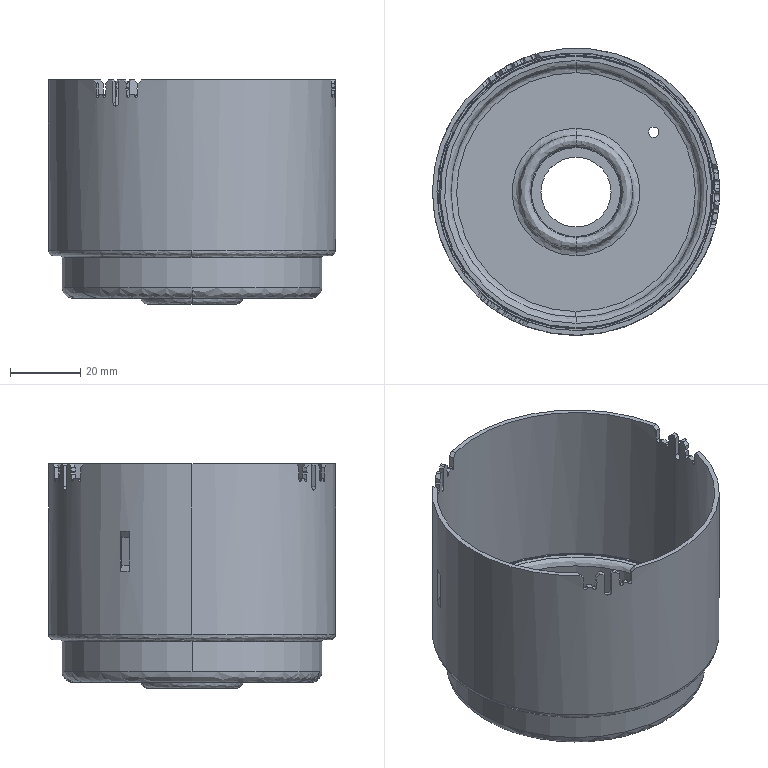Part | STEP file | TQ-DD-1105-THA140062100B_Housing1010_デフォルト | 1 solid | 157 faces | box 82 x 82 x 64.1 mm | volume 27832 mm3 | plane 86 | cylinder 45 | spline 26 | commonest cylinder face diameters 0.6 x12 1 x12 2 x3 3 x2 20 x2 26 x2